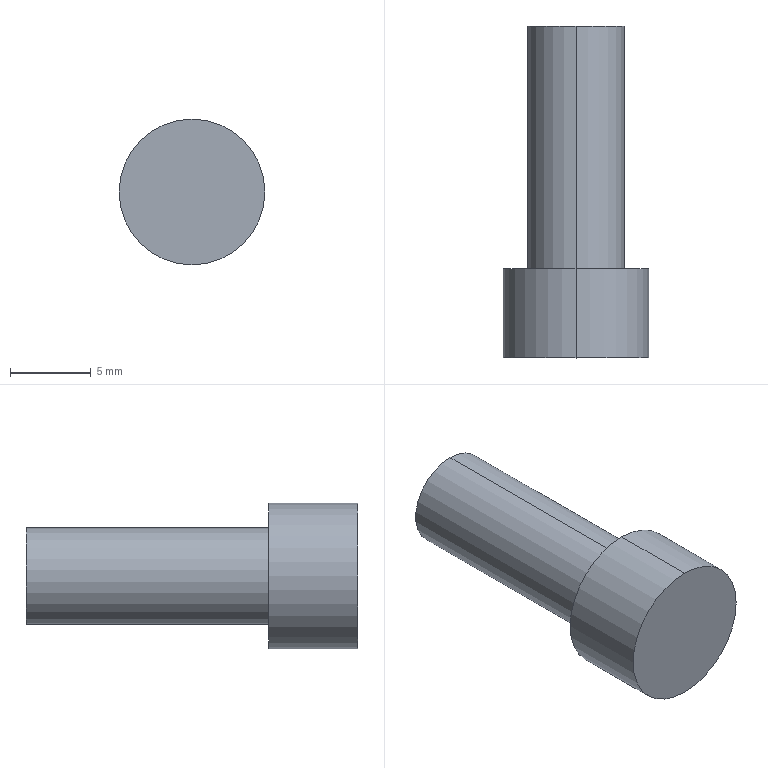Part | SolidWorks | features BaseBody 1 | 1 solid | 7 faces | box 9 x 20.5 x 9 mm | volume 774.01 mm3 | cylinder 4 | plane 3 | commonest cylinder face diameters 6 x2 9 x2
STEP:
#1=CARTESIAN_POINT('',(0.,0.,-4.5));
#2=VERTEX_POINT('',#1);
#3=CARTESIAN_POINT('',(0.,0.,4.5));
#4=VERTEX_POINT('',#3);
#5=CARTESIAN_POINT('',(0.,0.,0.));
#6=DIRECTION('',(0.,1.,0.));
#7=DIRECTION('',(0.,0.,-1.));
#8=AXIS2_PLACEMENT_3D('',#5,#6,#7);
#9=CIRCLE('',#8,4.5);
#10=EDGE_CURVE('',#2,#4,#9,.T.);
#11=ORIENTED_EDGE('',*,*,#10,.F.);
#12=CARTESIAN_POINT('',(0.,0.,0.));
#13=DIRECTION('',(0.,1.,0.));
#14=DIRECTION('',(0.,0.,-1.));
#15=AXIS2_PLACEMENT_3D('',#12,#13,#14);
#16=CIRCLE('',#15,4.5);
#17=EDGE_CURVE('',#4,#2,#16,.T.);
#18=ORIENTED_EDGE('',*,*,#17,.F.);
#19=EDGE_LOOP('',(#11,#18));
#20=FACE_OUTER_BOUND('',#19,.T.);
#21=CARTESIAN_POINT('',(0.,0.,0.));
#22=DIRECTION('',(0.,1.,0.));
#23=DIRECTION('',(1.,0.,0.));
#24=AXIS2_PLACEMENT_3D('',#21,#22,#23);
#25=PLANE('',#24);
#26=ADVANCED_FACE('',(#20),#25,.F.);
#27=CARTESIAN_POINT('',(0.,5.5,4.5));
#28=VERTEX_POINT('',#27);
#29=CARTESIAN_POINT('',(0.,5.5,4.5));
#30=DIRECTION('',(0.,-1.,0.));
#31=VECTOR('',#30,1000.);
#32=LINE('',#29,#31);
#33=EDGE_CURVE('',#28,#4,#32,.T.);
#34=ORIENTED_EDGE('',*,*,#33,.F.);
#35=CARTESIAN_POINT('',(0.,5.5,-4.5));
#36=VERTEX_POINT('',#35);
#37=CARTESIAN_POINT('',(0.,5.5,0.));
#38=DIRECTION('',(0.,1.,0.));
#39=DIRECTION('',(0.,0.,-1.));
#40=AXIS2_PLACEMENT_3D('',#37,#38,#39);
#41=CIRCLE('',#40,4.5);
#42=EDGE_CURVE('',#36,#28,#41,.T.);
#43=ORIENTED_EDGE('',*,*,#42,.F.);
#44=CARTESIAN_POINT('',(0.,5.5,-4.5));
#45=DIRECTION('',(0.,-1.,0.));
#46=VECTOR('',#45,1000.);
#47=LINE('',#44,#46);
#48=EDGE_CURVE('',#36,#2,#47,.T.);
#49=ORIENTED_EDGE('',*,*,#48,.T.);
#50=ORIENTED_EDGE('',*,*,#10,.T.);
#51=EDGE_LOOP('',(#34,#43,#49,#50));
#52=FACE_OUTER_BOUND('',#51,.T.);
#53=CARTESIAN_POINT('',(0.,5.5,0.));
#54=DIRECTION('',(0.,-1.,0.));
#55=DIRECTION('',(0.,0.,-1.));
#56=AXIS2_PLACEMENT_3D('',#53,#54,#55);
#57=CYLINDRICAL_SURFACE('',#56,4.5);
#58=ADVANCED_FACE('',(#52),#57,.T.);
#59=CARTESIAN_POINT('',(0.,20.5,-3.));
#60=VERTEX_POINT('',#59);
#61=CARTESIAN_POINT('',(0.,20.5,3.));
#62=VERTEX_POINT('',#61);
#63=CARTESIAN_POINT('',(0.,20.5,0.));
#64=DIRECTION('',(0.,-1.,0.));
#65=DIRECTION('',(0.,0.,-1.));
#66=AXIS2_PLACEMENT_3D('',#63,#64,#65);
#67=CIRCLE('',#66,3.);
#68=EDGE_CURVE('',#60,#62,#67,.T.);
#69=ORIENTED_EDGE('',*,*,#68,.F.);
#70=CARTESIAN_POINT('',(0.,20.5,0.));
#71=DIRECTION('',(0.,-1.,0.));
#72=DIRECTION('',(0.,0.,-1.));
#73=AXIS2_PLACEMENT_3D('',#70,#71,#72);
#74=CIRCLE('',#73,3.);
#75=EDGE_CURVE('',#62,#60,#74,.T.);
#76=ORIENTED_EDGE('',*,*,#75,.F.);
#77=EDGE_LOOP('',(#69,#76));
#78=FACE_OUTER_BOUND('',#77,.T.);
#79=CARTESIAN_POINT('',(0.,20.5,0.));
#80=DIRECTION('',(0.,1.,0.));
#81=DIRECTION('',(1.,0.,0.));
#82=AXIS2_PLACEMENT_3D('',#79,#80,#81);
#83=PLANE('',#82);
#84=ADVANCED_FACE('',(#78),#83,.T.);
#85=CARTESIAN_POINT('',(0.,5.5,-3.));
#86=VERTEX_POINT('',#85);
#87=CARTESIAN_POINT('',(0.,5.5,3.));
#88=VERTEX_POINT('',#87);
#89=CARTESIAN_POINT('',(0.,5.5,0.));
#90=DIRECTION('',(0.,1.,0.));
#91=DIRECTION('',(0.,0.,-1.));
#92=AXIS2_PLACEMENT_3D('',#89,#90,#91);
#93=CIRCLE('',#92,3.);
#94=EDGE_CURVE('',#86,#88,#93,.T.);
#95=ORIENTED_EDGE('',*,*,#94,.F.);
#96=CARTESIAN_POINT('',(0.,5.5,0.));
#97=DIRECTION('',(0.,1.,0.));
#98=DIRECTION('',(0.,0.,-1.));
#99=AXIS2_PLACEMENT_3D('',#96,#97,#98);
#100=CIRCLE('',#99,3.);
#101=EDGE_CURVE('',#88,#86,#100,.T.);
#102=ORIENTED_EDGE('',*,*,#101,.F.);
#103=EDGE_LOOP('',(#95,#102));
#104=FACE_BOUND('',#103,.T.);
#105=ORIENTED_EDGE('',*,*,#42,.T.);
#106=CARTESIAN_POINT('',(0.,5.5,0.));
#107=DIRECTION('',(0.,1.,0.));
#108=DIRECTION('',(0.,0.,-1.));
#109=AXIS2_PLACEMENT_3D('',#106,#107,#108);
#110=CIRCLE('',#109,4.5);
#111=EDGE_CURVE('',#28,#36,#110,.T.);
#112=ORIENTED_EDGE('',*,*,#111,.T.);
#113=EDGE_LOOP('',(#105,#112));
#114=FACE_OUTER_BOUND('',#113,.T.);
#115=CARTESIAN_POINT('',(0.,5.5,0.));
#116=DIRECTION('',(0.,1.,0.));
#117=DIRECTION('',(1.,0.,0.));
#118=AXIS2_PLACEMENT_3D('',#115,#116,#117);
#119=PLANE('',#118);
#120=ADVANCED_FACE('',(#104,#114),#119,.T.);
#121=CARTESIAN_POINT('',(0.,20.5,3.));
#122=DIRECTION('',(0.,-1.,0.));
#123=VECTOR('',#122,1000.);
#124=LINE('',#121,#123);
#125=EDGE_CURVE('',#62,#88,#124,.T.);
#126=ORIENTED_EDGE('',*,*,#125,.F.);
#127=ORIENTED_EDGE('',*,*,#75,.T.);
#128=CARTESIAN_POINT('',(0.,20.5,-3.));
#129=DIRECTION('',(0.,-1.,0.));
#130=VECTOR('',#129,1000.);
#131=LINE('',#128,#130);
#132=EDGE_CURVE('',#60,#86,#131,.T.);
#133=ORIENTED_EDGE('',*,*,#132,.T.);
#134=ORIENTED_EDGE('',*,*,#94,.T.);
#135=EDGE_LOOP('',(#126,#127,#133,#134));
#136=FACE_OUTER_BOUND('',#135,.T.);
#137=CARTESIAN_POINT('',(0.,20.5,0.));
#138=DIRECTION('',(0.,-1.,0.));
#139=DIRECTION('',(0.,0.,-1.));
#140=AXIS2_PLACEMENT_3D('',#137,#138,#139);
#141=CYLINDRICAL_SURFACE('',#140,3.);
#142=ADVANCED_FACE('',(#136),#141,.T.);
#143=ORIENTED_EDGE('',*,*,#111,.F.);
#144=ORIENTED_EDGE('',*,*,#33,.T.);
#145=ORIENTED_EDGE('',*,*,#17,.T.);
#146=ORIENTED_EDGE('',*,*,#48,.F.);
#147=EDGE_LOOP('',(#143,#144,#145,#146));
#148=FACE_OUTER_BOUND('',#147,.T.);
#149=CARTESIAN_POINT('',(0.,5.5,0.));
#150=DIRECTION('',(0.,-1.,0.));
#151=DIRECTION('',(0.,0.,-1.));
#152=AXIS2_PLACEMENT_3D('',#149,#150,#151);
#153=CYLINDRICAL_SURFACE('',#152,4.5);
#154=ADVANCED_FACE('',(#148),#153,.T.);
#155=ORIENTED_EDGE('',*,*,#68,.T.);
#156=ORIENTED_EDGE('',*,*,#125,.T.);
#157=ORIENTED_EDGE('',*,*,#101,.T.);
#158=ORIENTED_EDGE('',*,*,#132,.F.);
#159=EDGE_LOOP('',(#155,#156,#157,#158));
#160=FACE_OUTER_BOUND('',#159,.T.);
#161=CARTESIAN_POINT('',(0.,20.5,0.));
#162=DIRECTION('',(0.,-1.,0.));
#163=DIRECTION('',(0.,0.,-1.));
#164=AXIS2_PLACEMENT_3D('',#161,#162,#163);
#165=CYLINDRICAL_SURFACE('',#164,3.);
#166=ADVANCED_FACE('',(#160),#165,.T.);
#167=CLOSED_SHELL('',(#26,#58,#84,#120,#142,#154,#166));
#168=MANIFOLD_SOLID_BREP('',#167);
#169=CARTESIAN_POINT('',(0.,0.,0.));
#170=DIRECTION('',(0.,0.,1.));
#171=DIRECTION('',(1.,0.,0.));
#172=AXIS2_PLACEMENT_3D('',#169,#170,#171);
#173=(LENGTH_UNIT()NAMED_UNIT(*)SI_UNIT(.MILLI.,.METRE.));
#174=UNCERTAINTY_MEASURE_WITH_UNIT(LENGTH_MEASURE(0.00001),#173,'','');
#175=(NAMED_UNIT(*)PLANE_ANGLE_UNIT()SI_UNIT($,.RADIAN.));
#176=(NAMED_UNIT(*)SI_UNIT($,.STERADIAN.)SOLID_ANGLE_UNIT());
#177=(GEOMETRIC_REPRESENTATION_CONTEXT(3)GLOBAL_UNCERTAINTY_ASSIGNED_CONTEXT((#174))GLOBAL_UNIT_ASSIGNED_CONTEXT((#173,#175,#176))REPRESENTATION_CONTEXT('',''));
#178=ADVANCED_BREP_SHAPE_REPRESENTATION('',(#168,#172),#177);